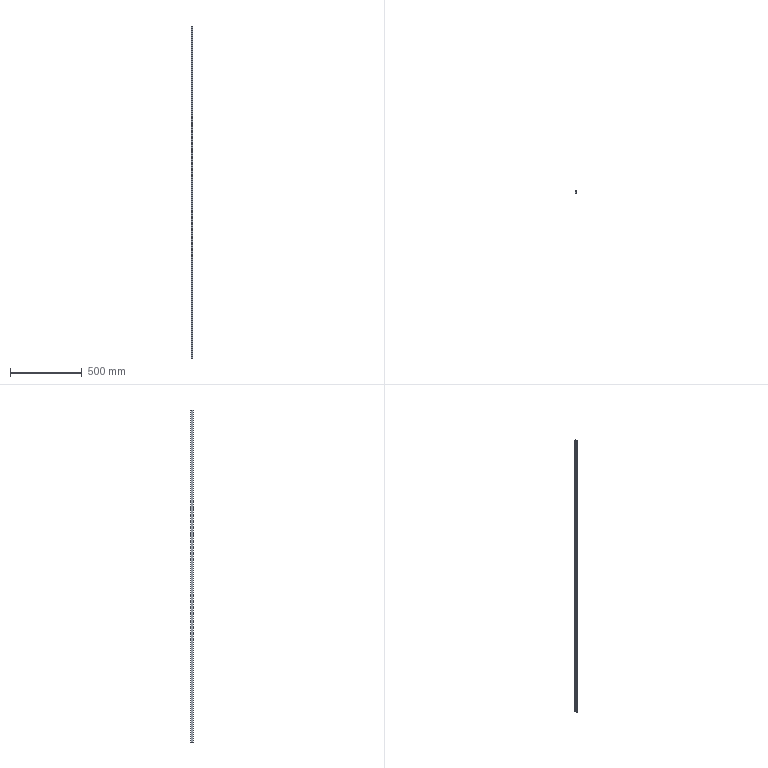Part | SolidWorks | features Extrusion 1 | 1 solid | 16 faces | box 8.5 x 18.686 x 2317 mm | volume 107612 mm3 | plane 16
STEP:
#1=CARTESIAN_POINT('',(7.255,-0.7862,0.));
#2=VERTEX_POINT('',#1);
#3=CARTESIAN_POINT('',(7.255,0.,0.));
#4=VERTEX_POINT('',#3);
#5=CARTESIAN_POINT('',(7.255,-0.7862,0.));
#6=DIRECTION('',(0.,1.,0.));
#7=VECTOR('',#6,1000.);
#8=LINE('',#5,#7);
#9=EDGE_CURVE('',#2,#4,#8,.T.);
#10=ORIENTED_EDGE('',*,*,#9,.T.);
#11=CARTESIAN_POINT('',(7.255,0.,2317.));
#12=VERTEX_POINT('',#11);
#13=CARTESIAN_POINT('',(7.255,0.,2317.));
#14=DIRECTION('',(0.,0.,-1.));
#15=VECTOR('',#14,1000.);
#16=LINE('',#13,#15);
#17=EDGE_CURVE('',#12,#4,#16,.T.);
#18=ORIENTED_EDGE('',*,*,#17,.F.);
#19=CARTESIAN_POINT('',(7.255,-0.7862,2317.));
#20=VERTEX_POINT('',#19);
#21=CARTESIAN_POINT('',(7.255,-0.7862,2317.));
#22=DIRECTION('',(0.,1.,0.));
#23=VECTOR('',#22,1000.);
#24=LINE('',#21,#23);
#25=EDGE_CURVE('',#20,#12,#24,.T.);
#26=ORIENTED_EDGE('',*,*,#25,.F.);
#27=CARTESIAN_POINT('',(7.255,-0.7862,2317.));
#28=DIRECTION('',(0.,0.,-1.));
#29=VECTOR('',#28,1000.);
#30=LINE('',#27,#29);
#31=EDGE_CURVE('',#20,#2,#30,.T.);
#32=ORIENTED_EDGE('',*,*,#31,.T.);
#33=EDGE_LOOP('',(#10,#18,#26,#32));
#34=FACE_OUTER_BOUND('',#33,.T.);
#35=CARTESIAN_POINT('',(7.255,-0.7862,2317.));
#36=DIRECTION('',(-1.,0.,0.));
#37=DIRECTION('',(0.,0.,1.));
#38=AXIS2_PLACEMENT_3D('',#35,#36,#37);
#39=PLANE('',#38);
#40=ADVANCED_FACE('',(#34),#39,.F.);
#41=CARTESIAN_POINT('',(3.255,0.,0.));
#42=VERTEX_POINT('',#41);
#43=CARTESIAN_POINT('',(7.255,0.,0.));
#44=DIRECTION('',(-1.,0.,0.));
#45=VECTOR('',#44,1000.);
#46=LINE('',#43,#45);
#47=EDGE_CURVE('',#4,#42,#46,.T.);
#48=ORIENTED_EDGE('',*,*,#47,.T.);
#49=CARTESIAN_POINT('',(3.255,0.,2317.));
#50=VERTEX_POINT('',#49);
#51=CARTESIAN_POINT('',(3.255,0.,2317.));
#52=DIRECTION('',(0.,0.,-1.));
#53=VECTOR('',#52,1000.);
#54=LINE('',#51,#53);
#55=EDGE_CURVE('',#50,#42,#54,.T.);
#56=ORIENTED_EDGE('',*,*,#55,.F.);
#57=CARTESIAN_POINT('',(7.255,0.,2317.));
#58=DIRECTION('',(-1.,0.,0.));
#59=VECTOR('',#58,1000.);
#60=LINE('',#57,#59);
#61=EDGE_CURVE('',#12,#50,#60,.T.);
#62=ORIENTED_EDGE('',*,*,#61,.F.);
#63=ORIENTED_EDGE('',*,*,#17,.T.);
#64=EDGE_LOOP('',(#48,#56,#62,#63));
#65=FACE_OUTER_BOUND('',#64,.T.);
#66=CARTESIAN_POINT('',(7.255,0.,2317.));
#67=DIRECTION('',(0.,-1.,0.));
#68=DIRECTION('',(1.,0.,0.));
#69=AXIS2_PLACEMENT_3D('',#66,#67,#68);
#70=PLANE('',#69);
#71=ADVANCED_FACE('',(#65),#70,.F.);
#72=CARTESIAN_POINT('',(3.255,-8.686,0.));
#73=VERTEX_POINT('',#72);
#74=CARTESIAN_POINT('',(3.255,0.,0.));
#75=DIRECTION('',(0.,-1.,0.));
#76=VECTOR('',#75,1000.);
#77=LINE('',#74,#76);
#78=EDGE_CURVE('',#42,#73,#77,.T.);
#79=ORIENTED_EDGE('',*,*,#78,.T.);
#80=CARTESIAN_POINT('',(3.255,-8.686,2317.));
#81=VERTEX_POINT('',#80);
#82=CARTESIAN_POINT('',(3.255,-8.686,2317.));
#83=DIRECTION('',(0.,0.,-1.));
#84=VECTOR('',#83,1000.);
#85=LINE('',#82,#84);
#86=EDGE_CURVE('',#81,#73,#85,.T.);
#87=ORIENTED_EDGE('',*,*,#86,.F.);
#88=CARTESIAN_POINT('',(3.255,0.,2317.));
#89=DIRECTION('',(0.,-1.,0.));
#90=VECTOR('',#89,1000.);
#91=LINE('',#88,#90);
#92=EDGE_CURVE('',#50,#81,#91,.T.);
#93=ORIENTED_EDGE('',*,*,#92,.F.);
#94=ORIENTED_EDGE('',*,*,#55,.T.);
#95=EDGE_LOOP('',(#79,#87,#93,#94));
#96=FACE_OUTER_BOUND('',#95,.T.);
#97=CARTESIAN_POINT('',(3.255,0.,2317.));
#98=DIRECTION('',(1.,0.,0.));
#99=DIRECTION('',(0.,1.,0.));
#100=AXIS2_PLACEMENT_3D('',#97,#98,#99);
#101=PLANE('',#100);
#102=ADVANCED_FACE('',(#96),#101,.F.);
#103=CARTESIAN_POINT('',(-0.2449,-8.686,0.));
#104=VERTEX_POINT('',#103);
#105=CARTESIAN_POINT('',(3.255,-8.686,0.));
#106=DIRECTION('',(-1.,0.,0.));
#107=VECTOR('',#106,1000.);
#108=LINE('',#105,#107);
#109=EDGE_CURVE('',#73,#104,#108,.T.);
#110=ORIENTED_EDGE('',*,*,#109,.T.);
#111=CARTESIAN_POINT('',(-0.2449,-8.686,2317.));
#112=VERTEX_POINT('',#111);
#113=CARTESIAN_POINT('',(-0.2449,-8.686,2317.));
#114=DIRECTION('',(0.,0.,-1.));
#115=VECTOR('',#114,1000.);
#116=LINE('',#113,#115);
#117=EDGE_CURVE('',#112,#104,#116,.T.);
#118=ORIENTED_EDGE('',*,*,#117,.F.);
#119=CARTESIAN_POINT('',(3.255,-8.686,2317.));
#120=DIRECTION('',(-1.,0.,0.));
#121=VECTOR('',#120,1000.);
#122=LINE('',#119,#121);
#123=EDGE_CURVE('',#81,#112,#122,.T.);
#124=ORIENTED_EDGE('',*,*,#123,.F.);
#125=ORIENTED_EDGE('',*,*,#86,.T.);
#126=EDGE_LOOP('',(#110,#118,#124,#125));
#127=FACE_OUTER_BOUND('',#126,.T.);
#128=CARTESIAN_POINT('',(3.255,-8.686,2317.));
#129=DIRECTION('',(0.,-1.,0.));
#130=DIRECTION('',(0.,0.,-1.));
#131=AXIS2_PLACEMENT_3D('',#128,#129,#130);
#132=PLANE('',#131);
#133=ADVANCED_FACE('',(#127),#132,.F.);
#134=CARTESIAN_POINT('',(-0.2449,0.,0.));
#135=VERTEX_POINT('',#134);
#136=CARTESIAN_POINT('',(-0.2449,-8.686,0.));
#137=DIRECTION('',(0.,1.,0.));
#138=VECTOR('',#137,1000.);
#139=LINE('',#136,#138);
#140=EDGE_CURVE('',#104,#135,#139,.T.);
#141=ORIENTED_EDGE('',*,*,#140,.T.);
#142=CARTESIAN_POINT('',(-0.2449,0.,2317.));
#143=VERTEX_POINT('',#142);
#144=CARTESIAN_POINT('',(-0.2449,0.,2317.));
#145=DIRECTION('',(0.,0.,-1.));
#146=VECTOR('',#145,1000.);
#147=LINE('',#144,#146);
#148=EDGE_CURVE('',#143,#135,#147,.T.);
#149=ORIENTED_EDGE('',*,*,#148,.F.);
#150=CARTESIAN_POINT('',(-0.2449,-8.686,2317.));
#151=DIRECTION('',(0.,1.,0.));
#152=VECTOR('',#151,1000.);
#153=LINE('',#150,#152);
#154=EDGE_CURVE('',#112,#143,#153,.T.);
#155=ORIENTED_EDGE('',*,*,#154,.F.);
#156=ORIENTED_EDGE('',*,*,#117,.T.);
#157=EDGE_LOOP('',(#141,#149,#155,#156));
#158=FACE_OUTER_BOUND('',#157,.T.);
#159=CARTESIAN_POINT('',(-0.2449,-8.686,2317.));
#160=DIRECTION('',(-1.,0.,0.));
#161=DIRECTION('',(0.,0.,1.));
#162=AXIS2_PLACEMENT_3D('',#159,#160,#161);
#163=PLANE('',#162);
#164=ADVANCED_FACE('',(#158),#163,.F.);
#165=CARTESIAN_POINT('',(-1.245,0.,0.));
#166=VERTEX_POINT('',#165);
#167=CARTESIAN_POINT('',(-0.2449,0.,0.));
#168=DIRECTION('',(-1.,0.,0.));
#169=VECTOR('',#168,1000.);
#170=LINE('',#167,#169);
#171=EDGE_CURVE('',#135,#166,#170,.T.);
#172=ORIENTED_EDGE('',*,*,#171,.T.);
#173=CARTESIAN_POINT('',(-1.245,0.,2317.));
#174=VERTEX_POINT('',#173);
#175=CARTESIAN_POINT('',(-1.245,0.,2317.));
#176=DIRECTION('',(0.,0.,-1.));
#177=VECTOR('',#176,1000.);
#178=LINE('',#175,#177);
#179=EDGE_CURVE('',#174,#166,#178,.T.);
#180=ORIENTED_EDGE('',*,*,#179,.F.);
#181=CARTESIAN_POINT('',(-0.2449,0.,2317.));
#182=DIRECTION('',(-1.,0.,0.));
#183=VECTOR('',#182,1000.);
#184=LINE('',#181,#183);
#185=EDGE_CURVE('',#143,#174,#184,.T.);
#186=ORIENTED_EDGE('',*,*,#185,.F.);
#187=ORIENTED_EDGE('',*,*,#148,.T.);
#188=EDGE_LOOP('',(#172,#180,#186,#187));
#189=FACE_OUTER_BOUND('',#188,.T.);
#190=CARTESIAN_POINT('',(-0.2449,0.,2317.));
#191=DIRECTION('',(0.,-1.,0.));
#192=DIRECTION('',(1.,0.,0.));
#193=AXIS2_PLACEMENT_3D('',#190,#191,#192);
#194=PLANE('',#193);
#195=ADVANCED_FACE('',(#189),#194,.F.);
#196=CARTESIAN_POINT('',(-1.245,-18.4,0.));
#197=VERTEX_POINT('',#196);
#198=CARTESIAN_POINT('',(-1.245,0.,0.));
#199=DIRECTION('',(0.,-1.,0.));
#200=VECTOR('',#199,1000.);
#201=LINE('',#198,#200);
#202=EDGE_CURVE('',#166,#197,#201,.T.);
#203=ORIENTED_EDGE('',*,*,#202,.T.);
#204=CARTESIAN_POINT('',(-1.245,-18.4,2317.));
#205=VERTEX_POINT('',#204);
#206=CARTESIAN_POINT('',(-1.245,-18.4,2317.));
#207=DIRECTION('',(0.,0.,-1.));
#208=VECTOR('',#207,1000.);
#209=LINE('',#206,#208);
#210=EDGE_CURVE('',#205,#197,#209,.T.);
#211=ORIENTED_EDGE('',*,*,#210,.F.);
#212=CARTESIAN_POINT('',(-1.245,0.,2317.));
#213=DIRECTION('',(0.,-1.,0.));
#214=VECTOR('',#213,1000.);
#215=LINE('',#212,#214);
#216=EDGE_CURVE('',#174,#205,#215,.T.);
#217=ORIENTED_EDGE('',*,*,#216,.F.);
#218=ORIENTED_EDGE('',*,*,#179,.T.);
#219=EDGE_LOOP('',(#203,#211,#217,#218));
#220=FACE_OUTER_BOUND('',#219,.T.);
#221=CARTESIAN_POINT('',(-1.245,0.,2317.));
#222=DIRECTION('',(1.,0.,0.));
#223=DIRECTION('',(0.,1.,0.));
#224=AXIS2_PLACEMENT_3D('',#221,#222,#223);
#225=PLANE('',#224);
#226=ADVANCED_FACE('',(#220),#225,.F.);
#227=CARTESIAN_POINT('',(-0.2449,-18.4,0.));
#228=VERTEX_POINT('',#227);
#229=CARTESIAN_POINT('',(-1.245,-18.4,0.));
#230=DIRECTION('',(1.,0.,0.));
#231=VECTOR('',#230,1000.);
#232=LINE('',#229,#231);
#233=EDGE_CURVE('',#197,#228,#232,.T.);
#234=ORIENTED_EDGE('',*,*,#233,.T.);
#235=CARTESIAN_POINT('',(-0.2449,-18.4,2317.));
#236=VERTEX_POINT('',#235);
#237=CARTESIAN_POINT('',(-0.2449,-18.4,2317.));
#238=DIRECTION('',(0.,0.,-1.));
#239=VECTOR('',#238,1000.);
#240=LINE('',#237,#239);
#241=EDGE_CURVE('',#236,#228,#240,.T.);
#242=ORIENTED_EDGE('',*,*,#241,.F.);
#243=CARTESIAN_POINT('',(-1.245,-18.4,2317.));
#244=DIRECTION('',(1.,0.,0.));
#245=VECTOR('',#244,1000.);
#246=LINE('',#243,#245);
#247=EDGE_CURVE('',#205,#236,#246,.T.);
#248=ORIENTED_EDGE('',*,*,#247,.F.);
#249=ORIENTED_EDGE('',*,*,#210,.T.);
#250=EDGE_LOOP('',(#234,#242,#248,#249));
#251=FACE_OUTER_BOUND('',#250,.T.);
#252=CARTESIAN_POINT('',(-1.245,-18.4,2317.));
#253=DIRECTION('',(0.,1.,0.));
#254=DIRECTION('',(0.,0.,1.));
#255=AXIS2_PLACEMENT_3D('',#252,#253,#254);
#256=PLANE('',#255);
#257=ADVANCED_FACE('',(#251),#256,.F.);
#258=CARTESIAN_POINT('',(-0.2449,-10.686,0.));
#259=VERTEX_POINT('',#258);
#260=CARTESIAN_POINT('',(-0.2449,-18.4,0.));
#261=DIRECTION('',(0.,1.,0.));
#262=VECTOR('',#261,1000.);
#263=LINE('',#260,#262);
#264=EDGE_CURVE('',#228,#259,#263,.T.);
#265=ORIENTED_EDGE('',*,*,#264,.T.);
#266=CARTESIAN_POINT('',(-0.2449,-10.686,2317.));
#267=VERTEX_POINT('',#266);
#268=CARTESIAN_POINT('',(-0.2449,-10.686,2317.));
#269=DIRECTION('',(0.,0.,-1.));
#270=VECTOR('',#269,1000.);
#271=LINE('',#268,#270);
#272=EDGE_CURVE('',#267,#259,#271,.T.);
#273=ORIENTED_EDGE('',*,*,#272,.F.);
#274=CARTESIAN_POINT('',(-0.2449,-18.4,2317.));
#275=DIRECTION('',(0.,1.,0.));
#276=VECTOR('',#275,1000.);
#277=LINE('',#274,#276);
#278=EDGE_CURVE('',#236,#267,#277,.T.);
#279=ORIENTED_EDGE('',*,*,#278,.F.);
#280=ORIENTED_EDGE('',*,*,#241,.T.);
#281=EDGE_LOOP('',(#265,#273,#279,#280));
#282=FACE_OUTER_BOUND('',#281,.T.);
#283=CARTESIAN_POINT('',(-0.2449,-18.4,2317.));
#284=DIRECTION('',(-1.,0.,0.));
#285=DIRECTION('',(0.,0.,1.));
#286=AXIS2_PLACEMENT_3D('',#283,#284,#285);
#287=PLANE('',#286);
#288=ADVANCED_FACE('',(#282),#287,.F.);
#289=CARTESIAN_POINT('',(3.255,-10.686,0.));
#290=VERTEX_POINT('',#289);
#291=CARTESIAN_POINT('',(-0.2449,-10.686,0.));
#292=DIRECTION('',(1.,0.,0.));
#293=VECTOR('',#292,1000.);
#294=LINE('',#291,#293);
#295=EDGE_CURVE('',#259,#290,#294,.T.);
#296=ORIENTED_EDGE('',*,*,#295,.T.);
#297=CARTESIAN_POINT('',(3.255,-10.686,2317.));
#298=VERTEX_POINT('',#297);
#299=CARTESIAN_POINT('',(3.255,-10.686,2317.));
#300=DIRECTION('',(0.,0.,-1.));
#301=VECTOR('',#300,1000.);
#302=LINE('',#299,#301);
#303=EDGE_CURVE('',#298,#290,#302,.T.);
#304=ORIENTED_EDGE('',*,*,#303,.F.);
#305=CARTESIAN_POINT('',(-0.2449,-10.686,2317.));
#306=DIRECTION('',(1.,0.,0.));
#307=VECTOR('',#306,1000.);
#308=LINE('',#305,#307);
#309=EDGE_CURVE('',#267,#298,#308,.T.);
#310=ORIENTED_EDGE('',*,*,#309,.F.);
#311=ORIENTED_EDGE('',*,*,#272,.T.);
#312=EDGE_LOOP('',(#296,#304,#310,#311));
#313=FACE_OUTER_BOUND('',#312,.T.);
#314=CARTESIAN_POINT('',(-0.2449,-10.686,2317.));
#315=DIRECTION('',(0.,1.,0.));
#316=DIRECTION('',(0.,0.,1.));
#317=AXIS2_PLACEMENT_3D('',#314,#315,#316);
#318=PLANE('',#317);
#319=ADVANCED_FACE('',(#313),#318,.F.);
#320=CARTESIAN_POINT('',(3.255,-18.686,0.));
#321=VERTEX_POINT('',#320);
#322=CARTESIAN_POINT('',(3.255,-10.686,0.));
#323=DIRECTION('',(0.,-1.,0.));
#324=VECTOR('',#323,1000.);
#325=LINE('',#322,#324);
#326=EDGE_CURVE('',#290,#321,#325,.T.);
#327=ORIENTED_EDGE('',*,*,#326,.T.);
#328=CARTESIAN_POINT('',(3.255,-18.686,2317.));
#329=VERTEX_POINT('',#328);
#330=CARTESIAN_POINT('',(3.255,-18.686,2317.));
#331=DIRECTION('',(0.,0.,-1.));
#332=VECTOR('',#331,1000.);
#333=LINE('',#330,#332);
#334=EDGE_CURVE('',#329,#321,#333,.T.);
#335=ORIENTED_EDGE('',*,*,#334,.F.);
#336=CARTESIAN_POINT('',(3.255,-10.686,2317.));
#337=DIRECTION('',(0.,-1.,0.));
#338=VECTOR('',#337,1000.);
#339=LINE('',#336,#338);
#340=EDGE_CURVE('',#298,#329,#339,.T.);
#341=ORIENTED_EDGE('',*,*,#340,.F.);
#342=ORIENTED_EDGE('',*,*,#303,.T.);
#343=EDGE_LOOP('',(#327,#335,#341,#342));
#344=FACE_OUTER_BOUND('',#343,.T.);
#345=CARTESIAN_POINT('',(3.255,-10.686,2317.));
#346=DIRECTION('',(1.,0.,0.));
#347=DIRECTION('',(0.,1.,0.));
#348=AXIS2_PLACEMENT_3D('',#345,#346,#347);
#349=PLANE('',#348);
#350=ADVANCED_FACE('',(#344),#349,.F.);
#351=CARTESIAN_POINT('',(4.255,-18.686,0.));
#352=VERTEX_POINT('',#351);
#353=CARTESIAN_POINT('',(3.255,-18.686,0.));
#354=DIRECTION('',(1.,0.,0.));
#355=VECTOR('',#354,1000.);
#356=LINE('',#353,#355);
#357=EDGE_CURVE('',#321,#352,#356,.T.);
#358=ORIENTED_EDGE('',*,*,#357,.T.);
#359=CARTESIAN_POINT('',(4.255,-18.686,2317.));
#360=VERTEX_POINT('',#359);
#361=CARTESIAN_POINT('',(4.255,-18.686,2317.));
#362=DIRECTION('',(0.,0.,-1.));
#363=VECTOR('',#362,1000.);
#364=LINE('',#361,#363);
#365=EDGE_CURVE('',#360,#352,#364,.T.);
#366=ORIENTED_EDGE('',*,*,#365,.F.);
#367=CARTESIAN_POINT('',(3.255,-18.686,2317.));
#368=DIRECTION('',(1.,0.,0.));
#369=VECTOR('',#368,1000.);
#370=LINE('',#367,#369);
#371=EDGE_CURVE('',#329,#360,#370,.T.);
#372=ORIENTED_EDGE('',*,*,#371,.F.);
#373=ORIENTED_EDGE('',*,*,#334,.T.);
#374=EDGE_LOOP('',(#358,#366,#372,#373));
#375=FACE_OUTER_BOUND('',#374,.T.);
#376=CARTESIAN_POINT('',(3.255,-18.686,2317.));
#377=DIRECTION('',(0.,1.,0.));
#378=DIRECTION('',(0.,0.,1.));
#379=AXIS2_PLACEMENT_3D('',#376,#377,#378);
#380=PLANE('',#379);
#381=ADVANCED_FACE('',(#375),#380,.F.);
#382=CARTESIAN_POINT('',(4.255,-0.7862,0.));
#383=VERTEX_POINT('',#382);
#384=CARTESIAN_POINT('',(4.255,-18.686,0.));
#385=DIRECTION('',(0.,1.,0.));
#386=VECTOR('',#385,1000.);
#387=LINE('',#384,#386);
#388=EDGE_CURVE('',#352,#383,#387,.T.);
#389=ORIENTED_EDGE('',*,*,#388,.T.);
#390=CARTESIAN_POINT('',(4.255,-0.7862,2317.));
#391=VERTEX_POINT('',#390);
#392=CARTESIAN_POINT('',(4.255,-0.7862,2317.));
#393=DIRECTION('',(0.,0.,-1.));
#394=VECTOR('',#393,1000.);
#395=LINE('',#392,#394);
#396=EDGE_CURVE('',#391,#383,#395,.T.);
#397=ORIENTED_EDGE('',*,*,#396,.F.);
#398=CARTESIAN_POINT('',(4.255,-18.686,2317.));
#399=DIRECTION('',(0.,1.,0.));
#400=VECTOR('',#399,1000.);
#401=LINE('',#398,#400);
#402=EDGE_CURVE('',#360,#391,#401,.T.);
#403=ORIENTED_EDGE('',*,*,#402,.F.);
#404=ORIENTED_EDGE('',*,*,#365,.T.);
#405=EDGE_LOOP('',(#389,#397,#403,#404));
#406=FACE_OUTER_BOUND('',#405,.T.);
#407=CARTESIAN_POINT('',(4.255,-18.686,2317.));
#408=DIRECTION('',(-1.,0.,0.));
#409=DIRECTION('',(0.,0.,1.));
#410=AXIS2_PLACEMENT_3D('',#407,#408,#409);
#411=PLANE('',#410);
#412=ADVANCED_FACE('',(#406),#411,.F.);
#413=CARTESIAN_POINT('',(4.255,-0.7862,0.));
#414=DIRECTION('',(1.,0.,0.));
#415=VECTOR('',#414,1000.);
#416=LINE('',#413,#415);
#417=EDGE_CURVE('',#383,#2,#416,.T.);
#418=ORIENTED_EDGE('',*,*,#417,.T.);
#419=ORIENTED_EDGE('',*,*,#31,.F.);
#420=CARTESIAN_POINT('',(4.255,-0.7862,2317.));
#421=DIRECTION('',(1.,0.,0.));
#422=VECTOR('',#421,1000.);
#423=LINE('',#420,#422);
#424=EDGE_CURVE('',#391,#20,#423,.T.);
#425=ORIENTED_EDGE('',*,*,#424,.F.);
#426=ORIENTED_EDGE('',*,*,#396,.T.);
#427=EDGE_LOOP('',(#418,#419,#425,#426));
#428=FACE_OUTER_BOUND('',#427,.T.);
#429=CARTESIAN_POINT('',(4.255,-0.7862,2317.));
#430=DIRECTION('',(0.,1.,0.));
#431=DIRECTION('',(0.,0.,1.));
#432=AXIS2_PLACEMENT_3D('',#429,#430,#431);
#433=PLANE('',#432);
#434=ADVANCED_FACE('',(#428),#433,.F.);
#435=ORIENTED_EDGE('',*,*,#25,.T.);
#436=ORIENTED_EDGE('',*,*,#61,.T.);
#437=ORIENTED_EDGE('',*,*,#92,.T.);
#438=ORIENTED_EDGE('',*,*,#123,.T.);
#439=ORIENTED_EDGE('',*,*,#154,.T.);
#440=ORIENTED_EDGE('',*,*,#185,.T.);
#441=ORIENTED_EDGE('',*,*,#216,.T.);
#442=ORIENTED_EDGE('',*,*,#247,.T.);
#443=ORIENTED_EDGE('',*,*,#278,.T.);
#444=ORIENTED_EDGE('',*,*,#309,.T.);
#445=ORIENTED_EDGE('',*,*,#340,.T.);
#446=ORIENTED_EDGE('',*,*,#371,.T.);
#447=ORIENTED_EDGE('',*,*,#402,.T.);
#448=ORIENTED_EDGE('',*,*,#424,.T.);
#449=EDGE_LOOP('',(#435,#436,#437,#438,#439,#440,#441,#442,#443,#444,#445,#446,#447,#448));
#450=FACE_OUTER_BOUND('',#449,.T.);
#451=CARTESIAN_POINT('',(0.,0.,2317.));
#452=DIRECTION('',(0.,0.,1.));
#453=DIRECTION('',(1.,0.,0.));
#454=AXIS2_PLACEMENT_3D('',#451,#452,#453);
#455=PLANE('',#454);
#456=ADVANCED_FACE('',(#450),#455,.T.);
#457=ORIENTED_EDGE('',*,*,#9,.F.);
#458=ORIENTED_EDGE('',*,*,#417,.F.);
#459=ORIENTED_EDGE('',*,*,#388,.F.);
#460=ORIENTED_EDGE('',*,*,#357,.F.);
#461=ORIENTED_EDGE('',*,*,#326,.F.);
#462=ORIENTED_EDGE('',*,*,#295,.F.);
#463=ORIENTED_EDGE('',*,*,#264,.F.);
#464=ORIENTED_EDGE('',*,*,#233,.F.);
#465=ORIENTED_EDGE('',*,*,#202,.F.);
#466=ORIENTED_EDGE('',*,*,#171,.F.);
#467=ORIENTED_EDGE('',*,*,#140,.F.);
#468=ORIENTED_EDGE('',*,*,#109,.F.);
#469=ORIENTED_EDGE('',*,*,#78,.F.);
#470=ORIENTED_EDGE('',*,*,#47,.F.);
#471=EDGE_LOOP('',(#457,#458,#459,#460,#461,#462,#463,#464,#465,#466,#467,#468,#469,#470));
#472=FACE_OUTER_BOUND('',#471,.T.);
#473=CARTESIAN_POINT('',(0.,0.,0.));
#474=DIRECTION('',(0.,0.,1.));
#475=DIRECTION('',(1.,0.,0.));
#476=AXIS2_PLACEMENT_3D('',#473,#474,#475);
#477=PLANE('',#476);
#478=ADVANCED_FACE('',(#472),#477,.F.);
#479=CLOSED_SHELL('',(#40,#71,#102,#133,#164,#195,#226,#257,#288,#319,#350,#381,#412,#434,#456,#478));
#480=MANIFOLD_SOLID_BREP('',#479);
#481=CARTESIAN_POINT('',(0.,0.,0.));
#482=DIRECTION('',(0.,0.,1.));
#483=DIRECTION('',(1.,0.,0.));
#484=AXIS2_PLACEMENT_3D('',#481,#482,#483);
#485=(LENGTH_UNIT()NAMED_UNIT(*)SI_UNIT(.MILLI.,.METRE.));
#486=UNCERTAINTY_MEASURE_WITH_UNIT(LENGTH_MEASURE(0.00001),#485,'','');
#487=(NAMED_UNIT(*)PLANE_ANGLE_UNIT()SI_UNIT($,.RADIAN.));
#488=(NAMED_UNIT(*)SI_UNIT($,.STERADIAN.)SOLID_ANGLE_UNIT());
#489=(GEOMETRIC_REPRESENTATION_CONTEXT(3)GLOBAL_UNCERTAINTY_ASSIGNED_CONTEXT((#486))GLOBAL_UNIT_ASSIGNED_CONTEXT((#485,#487,#488))REPRESENTATION_CONTEXT('',''));
#490=ADVANCED_BREP_SHAPE_REPRESENTATION('',(#480,#484),#489);